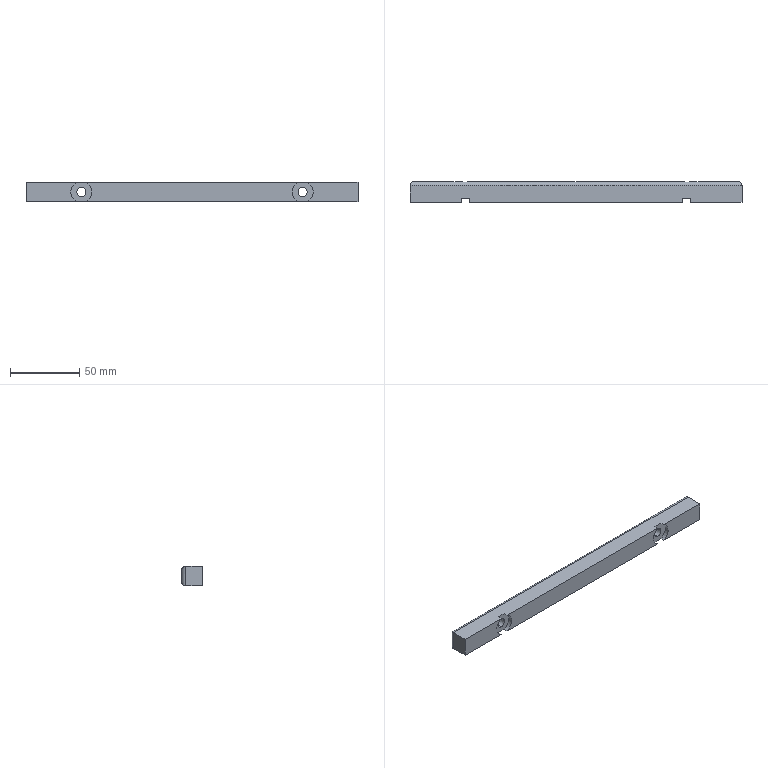Part | STEP file | PN_0006 | 1 solid | 30 faces | box 240 x 15 x 14 mm | volume 46724 mm3 | cylinder 16 | plane 14 | commonest cylinder face diameters 6 x4 6.6 x4 11 x4 15.2 x4